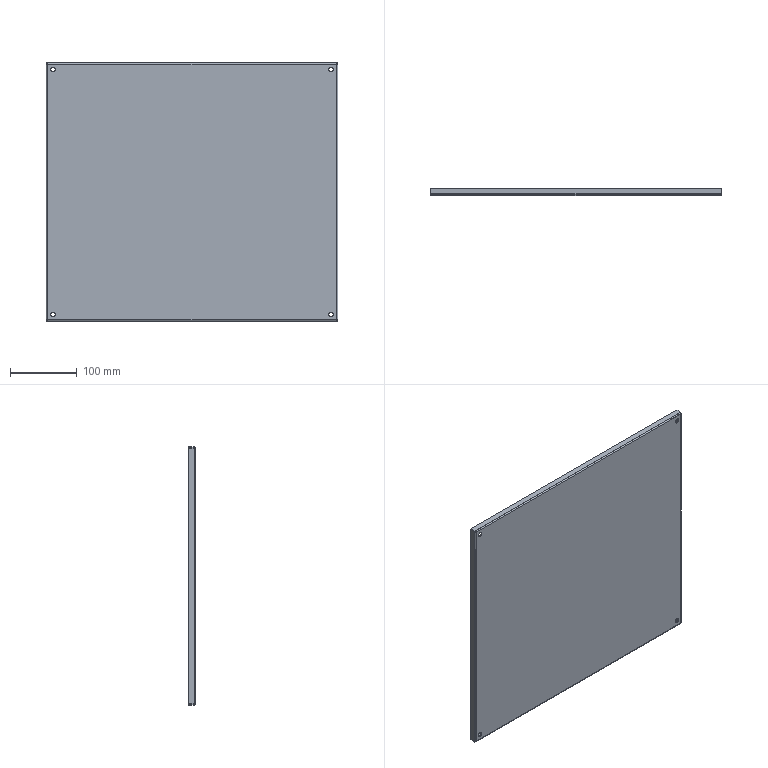Part | SolidWorks | features BaseBody 1 | 1 solid | 46 faces | box 436 x 10 x 386 mm | volume 272050 mm3 | plane 30 | cylinder 16 | commonest cylinder face diameters 7 x8 0.4 x4 3.4 x4
STEP:
#1=CARTESIAN_POINT('',(1238.,514.5,404.5));
#2=VERTEX_POINT('',#1);
#3=CARTESIAN_POINT('',(1238.,514.5,411.5));
#4=VERTEX_POINT('',#3);
#5=CARTESIAN_POINT('',(1238.,514.5,408.));
#6=DIRECTION('',(0.,1.,0.));
#7=DIRECTION('',(0.,0.,1.));
#8=AXIS2_PLACEMENT_3D('',#5,#6,#7);
#9=CIRCLE('',#8,3.5);
#10=EDGE_CURVE('',#2,#4,#9,.T.);
#11=ORIENTED_EDGE('',*,*,#10,.T.);
#12=CARTESIAN_POINT('',(1238.,513.,411.5));
#13=VERTEX_POINT('',#12);
#14=CARTESIAN_POINT('',(1238.,513.,411.5));
#15=DIRECTION('',(0.,-1.,0.));
#16=VECTOR('',#15,1000.);
#17=LINE('',#14,#16);
#18=EDGE_CURVE('',#4,#13,#17,.T.);
#19=ORIENTED_EDGE('',*,*,#18,.T.);
#20=CARTESIAN_POINT('',(1238.,513.,404.5));
#21=VERTEX_POINT('',#20);
#22=CARTESIAN_POINT('',(1238.,513.,408.));
#23=DIRECTION('',(0.,-1.,0.));
#24=DIRECTION('',(0.,0.,1.));
#25=AXIS2_PLACEMENT_3D('',#22,#23,#24);
#26=CIRCLE('',#25,3.5);
#27=EDGE_CURVE('',#13,#21,#26,.T.);
#28=ORIENTED_EDGE('',*,*,#27,.T.);
#29=CARTESIAN_POINT('',(1238.,513.,404.5));
#30=DIRECTION('',(0.,-1.,0.));
#31=VECTOR('',#30,1000.);
#32=LINE('',#29,#31);
#33=EDGE_CURVE('',#2,#21,#32,.T.);
#34=ORIENTED_EDGE('',*,*,#33,.F.);
#35=EDGE_LOOP('',(#11,#19,#28,#34));
#36=FACE_OUTER_BOUND('',#35,.T.);
#37=CARTESIAN_POINT('',(1238.,513.,408.));
#38=DIRECTION('',(0.,-1.,0.));
#39=DIRECTION('',(0.,0.,-1.));
#40=AXIS2_PLACEMENT_3D('',#37,#38,#39);
#41=CYLINDRICAL_SURFACE('',#40,3.5);
#42=ADVANCED_FACE('',(#36),#41,.F.);
#43=CARTESIAN_POINT('',(822.,514.5,38.5));
#44=VERTEX_POINT('',#43);
#45=CARTESIAN_POINT('',(822.,514.5,45.5));
#46=VERTEX_POINT('',#45);
#47=CARTESIAN_POINT('',(822.,514.5,42.));
#48=DIRECTION('',(0.,1.,0.));
#49=DIRECTION('',(0.,0.,1.));
#50=AXIS2_PLACEMENT_3D('',#47,#48,#49);
#51=CIRCLE('',#50,3.5);
#52=EDGE_CURVE('',#44,#46,#51,.T.);
#53=ORIENTED_EDGE('',*,*,#52,.T.);
#54=CARTESIAN_POINT('',(822.,513.,45.5));
#55=VERTEX_POINT('',#54);
#56=CARTESIAN_POINT('',(822.,513.,45.5));
#57=DIRECTION('',(0.,-1.,0.));
#58=VECTOR('',#57,1000.);
#59=LINE('',#56,#58);
#60=EDGE_CURVE('',#46,#55,#59,.T.);
#61=ORIENTED_EDGE('',*,*,#60,.T.);
#62=CARTESIAN_POINT('',(822.,513.,38.5));
#63=VERTEX_POINT('',#62);
#64=CARTESIAN_POINT('',(822.,513.,42.));
#65=DIRECTION('',(0.,-1.,0.));
#66=DIRECTION('',(0.,0.,1.));
#67=AXIS2_PLACEMENT_3D('',#64,#65,#66);
#68=CIRCLE('',#67,3.5);
#69=EDGE_CURVE('',#55,#63,#68,.T.);
#70=ORIENTED_EDGE('',*,*,#69,.T.);
#71=CARTESIAN_POINT('',(822.,513.,38.5));
#72=DIRECTION('',(0.,-1.,0.));
#73=VECTOR('',#72,1000.);
#74=LINE('',#71,#73);
#75=EDGE_CURVE('',#44,#63,#74,.T.);
#76=ORIENTED_EDGE('',*,*,#75,.F.);
#77=EDGE_LOOP('',(#53,#61,#70,#76));
#78=FACE_OUTER_BOUND('',#77,.T.);
#79=CARTESIAN_POINT('',(822.,513.,42.));
#80=DIRECTION('',(0.,-1.,0.));
#81=DIRECTION('',(0.,0.,-1.));
#82=AXIS2_PLACEMENT_3D('',#79,#80,#81);
#83=CYLINDRICAL_SURFACE('',#82,3.5);
#84=ADVANCED_FACE('',(#78),#83,.F.);
#85=CARTESIAN_POINT('',(822.,514.5,404.5));
#86=VERTEX_POINT('',#85);
#87=CARTESIAN_POINT('',(822.,514.5,411.5));
#88=VERTEX_POINT('',#87);
#89=CARTESIAN_POINT('',(822.,514.5,408.));
#90=DIRECTION('',(0.,1.,0.));
#91=DIRECTION('',(0.,0.,1.));
#92=AXIS2_PLACEMENT_3D('',#89,#90,#91);
#93=CIRCLE('',#92,3.5);
#94=EDGE_CURVE('',#86,#88,#93,.T.);
#95=ORIENTED_EDGE('',*,*,#94,.T.);
#96=CARTESIAN_POINT('',(822.,513.,411.5));
#97=VERTEX_POINT('',#96);
#98=CARTESIAN_POINT('',(822.,513.,411.5));
#99=DIRECTION('',(0.,-1.,0.));
#100=VECTOR('',#99,1000.);
#101=LINE('',#98,#100);
#102=EDGE_CURVE('',#88,#97,#101,.T.);
#103=ORIENTED_EDGE('',*,*,#102,.T.);
#104=CARTESIAN_POINT('',(822.,513.,404.5));
#105=VERTEX_POINT('',#104);
#106=CARTESIAN_POINT('',(822.,513.,408.));
#107=DIRECTION('',(0.,-1.,0.));
#108=DIRECTION('',(0.,0.,1.));
#109=AXIS2_PLACEMENT_3D('',#106,#107,#108);
#110=CIRCLE('',#109,3.5);
#111=EDGE_CURVE('',#97,#105,#110,.T.);
#112=ORIENTED_EDGE('',*,*,#111,.T.);
#113=CARTESIAN_POINT('',(822.,513.,404.5));
#114=DIRECTION('',(0.,-1.,0.));
#115=VECTOR('',#114,1000.);
#116=LINE('',#113,#115);
#117=EDGE_CURVE('',#86,#105,#116,.T.);
#118=ORIENTED_EDGE('',*,*,#117,.F.);
#119=EDGE_LOOP('',(#95,#103,#112,#118));
#120=FACE_OUTER_BOUND('',#119,.T.);
#121=CARTESIAN_POINT('',(822.,513.,408.));
#122=DIRECTION('',(0.,-1.,0.));
#123=DIRECTION('',(0.,0.,-1.));
#124=AXIS2_PLACEMENT_3D('',#121,#122,#123);
#125=CYLINDRICAL_SURFACE('',#124,3.5);
#126=ADVANCED_FACE('',(#120),#125,.F.);
#127=CARTESIAN_POINT('',(1238.,514.5,38.5));
#128=VERTEX_POINT('',#127);
#129=CARTESIAN_POINT('',(1238.,514.5,45.5));
#130=VERTEX_POINT('',#129);
#131=CARTESIAN_POINT('',(1238.,514.5,42.));
#132=DIRECTION('',(0.,1.,0.));
#133=DIRECTION('',(0.,0.,1.));
#134=AXIS2_PLACEMENT_3D('',#131,#132,#133);
#135=CIRCLE('',#134,3.5);
#136=EDGE_CURVE('',#128,#130,#135,.T.);
#137=ORIENTED_EDGE('',*,*,#136,.T.);
#138=CARTESIAN_POINT('',(1238.,513.,45.5));
#139=VERTEX_POINT('',#138);
#140=CARTESIAN_POINT('',(1238.,513.,45.5));
#141=DIRECTION('',(0.,-1.,0.));
#142=VECTOR('',#141,1000.);
#143=LINE('',#140,#142);
#144=EDGE_CURVE('',#130,#139,#143,.T.);
#145=ORIENTED_EDGE('',*,*,#144,.T.);
#146=CARTESIAN_POINT('',(1238.,513.,38.5));
#147=VERTEX_POINT('',#146);
#148=CARTESIAN_POINT('',(1238.,513.,42.));
#149=DIRECTION('',(0.,-1.,0.));
#150=DIRECTION('',(0.,0.,1.));
#151=AXIS2_PLACEMENT_3D('',#148,#149,#150);
#152=CIRCLE('',#151,3.5);
#153=EDGE_CURVE('',#139,#147,#152,.T.);
#154=ORIENTED_EDGE('',*,*,#153,.T.);
#155=CARTESIAN_POINT('',(1238.,513.,38.5));
#156=DIRECTION('',(0.,-1.,0.));
#157=VECTOR('',#156,1000.);
#158=LINE('',#155,#157);
#159=EDGE_CURVE('',#128,#147,#158,.T.);
#160=ORIENTED_EDGE('',*,*,#159,.F.);
#161=EDGE_LOOP('',(#137,#145,#154,#160));
#162=FACE_OUTER_BOUND('',#161,.T.);
#163=CARTESIAN_POINT('',(1238.,513.,42.));
#164=DIRECTION('',(0.,-1.,0.));
#165=DIRECTION('',(0.,0.,-1.));
#166=AXIS2_PLACEMENT_3D('',#163,#164,#165);
#167=CYLINDRICAL_SURFACE('',#166,3.5);
#168=ADVANCED_FACE('',(#162),#167,.F.);
#169=CARTESIAN_POINT('',(1246.5,514.7,416.));
#170=VERTEX_POINT('',#169);
#171=CARTESIAN_POINT('',(1246.3,514.5,416.));
#172=VERTEX_POINT('',#171);
#173=CARTESIAN_POINT('',(1246.3,514.7,416.));
#174=DIRECTION('',(0.,0.,-1.));
#175=DIRECTION('',(-1.,0.,0.));
#176=AXIS2_PLACEMENT_3D('',#173,#174,#175);
#177=CIRCLE('',#176,0.2);
#178=EDGE_CURVE('',#170,#172,#177,.T.);
#179=ORIENTED_EDGE('',*,*,#178,.F.);
#180=CARTESIAN_POINT('',(1246.5,514.7,34.));
#181=VERTEX_POINT('',#180);
#182=CARTESIAN_POINT('',(1246.5,514.7,421.));
#183=DIRECTION('',(0.,0.,1.));
#184=VECTOR('',#183,1000.);
#185=LINE('',#182,#184);
#186=EDGE_CURVE('',#181,#170,#185,.T.);
#187=ORIENTED_EDGE('',*,*,#186,.F.);
#188=CARTESIAN_POINT('',(1246.3,514.5,34.));
#189=VERTEX_POINT('',#188);
#190=CARTESIAN_POINT('',(1246.3,514.7,34.));
#191=DIRECTION('',(0.,0.,1.));
#192=DIRECTION('',(-1.,0.,0.));
#193=AXIS2_PLACEMENT_3D('',#190,#191,#192);
#194=CIRCLE('',#193,0.2);
#195=EDGE_CURVE('',#189,#181,#194,.T.);
#196=ORIENTED_EDGE('',*,*,#195,.F.);
#197=CARTESIAN_POINT('',(1246.3,514.5,421.));
#198=DIRECTION('',(0.,0.,-1.));
#199=VECTOR('',#198,1000.);
#200=LINE('',#197,#199);
#201=EDGE_CURVE('',#172,#189,#200,.T.);
#202=ORIENTED_EDGE('',*,*,#201,.F.);
#203=EDGE_LOOP('',(#179,#187,#196,#202));
#204=FACE_OUTER_BOUND('',#203,.T.);
#205=CARTESIAN_POINT('',(1246.3,514.7,1003.962));
#206=DIRECTION('',(0.,0.,-1.));
#207=DIRECTION('',(-1.,0.,0.));
#208=AXIS2_PLACEMENT_3D('',#205,#206,#207);
#209=CYLINDRICAL_SURFACE('',#208,0.2);
#210=ADVANCED_FACE('',(#204),#209,.F.);
#211=CARTESIAN_POINT('',(1248.,514.7,416.));
#212=VERTEX_POINT('',#211);
#213=CARTESIAN_POINT('',(1246.3,513.,416.));
#214=VERTEX_POINT('',#213);
#215=CARTESIAN_POINT('',(1246.3,514.7,416.));
#216=DIRECTION('',(0.,0.,-1.));
#217=DIRECTION('',(-1.,0.,0.));
#218=AXIS2_PLACEMENT_3D('',#215,#216,#217);
#219=CIRCLE('',#218,1.7);
#220=EDGE_CURVE('',#212,#214,#219,.T.);
#221=ORIENTED_EDGE('',*,*,#220,.T.);
#222=CARTESIAN_POINT('',(1246.3,513.,34.));
#223=VERTEX_POINT('',#222);
#224=CARTESIAN_POINT('',(1246.3,513.,421.));
#225=DIRECTION('',(0.,0.,-1.));
#226=VECTOR('',#225,1000.);
#227=LINE('',#224,#226);
#228=EDGE_CURVE('',#214,#223,#227,.T.);
#229=ORIENTED_EDGE('',*,*,#228,.T.);
#230=CARTESIAN_POINT('',(1248.,514.7,34.));
#231=VERTEX_POINT('',#230);
#232=CARTESIAN_POINT('',(1246.3,514.7,34.));
#233=DIRECTION('',(0.,0.,1.));
#234=DIRECTION('',(-1.,0.,0.));
#235=AXIS2_PLACEMENT_3D('',#232,#233,#234);
#236=CIRCLE('',#235,1.7);
#237=EDGE_CURVE('',#223,#231,#236,.T.);
#238=ORIENTED_EDGE('',*,*,#237,.T.);
#239=CARTESIAN_POINT('',(1248.,514.7,421.));
#240=DIRECTION('',(0.,0.,1.));
#241=VECTOR('',#240,1000.);
#242=LINE('',#239,#241);
#243=EDGE_CURVE('',#231,#212,#242,.T.);
#244=ORIENTED_EDGE('',*,*,#243,.T.);
#245=EDGE_LOOP('',(#221,#229,#238,#244));
#246=FACE_OUTER_BOUND('',#245,.T.);
#247=CARTESIAN_POINT('',(1246.3,514.7,1003.962));
#248=DIRECTION('',(0.,0.,-1.));
#249=DIRECTION('',(-1.,0.,0.));
#250=AXIS2_PLACEMENT_3D('',#247,#248,#249);
#251=CYLINDRICAL_SURFACE('',#250,1.7);
#252=ADVANCED_FACE('',(#246),#251,.T.);
#253=CARTESIAN_POINT('',(1246.,514.7,33.5));
#254=VERTEX_POINT('',#253);
#255=CARTESIAN_POINT('',(1246.,514.5,33.7));
#256=VERTEX_POINT('',#255);
#257=CARTESIAN_POINT('',(1246.,514.7,33.7));
#258=DIRECTION('',(-1.,0.,0.));
#259=DIRECTION('',(0.,0.,1.));
#260=AXIS2_PLACEMENT_3D('',#257,#258,#259);
#261=CIRCLE('',#260,0.2);
#262=EDGE_CURVE('',#254,#256,#261,.T.);
#263=ORIENTED_EDGE('',*,*,#262,.F.);
#264=CARTESIAN_POINT('',(814.,514.7,33.5));
#265=VERTEX_POINT('',#264);
#266=CARTESIAN_POINT('',(1251.,514.7,33.5));
#267=DIRECTION('',(1.,0.,0.));
#268=VECTOR('',#267,1000.);
#269=LINE('',#266,#268);
#270=EDGE_CURVE('',#265,#254,#269,.T.);
#271=ORIENTED_EDGE('',*,*,#270,.F.);
#272=CARTESIAN_POINT('',(814.,514.5,33.7));
#273=VERTEX_POINT('',#272);
#274=CARTESIAN_POINT('',(814.,514.7,33.7));
#275=DIRECTION('',(1.,0.,0.));
#276=DIRECTION('',(0.,0.,1.));
#277=AXIS2_PLACEMENT_3D('',#274,#275,#276);
#278=CIRCLE('',#277,0.2);
#279=EDGE_CURVE('',#273,#265,#278,.T.);
#280=ORIENTED_EDGE('',*,*,#279,.F.);
#281=CARTESIAN_POINT('',(1251.,514.5,33.7));
#282=DIRECTION('',(-1.,0.,0.));
#283=VECTOR('',#282,1000.);
#284=LINE('',#281,#283);
#285=EDGE_CURVE('',#256,#273,#284,.T.);
#286=ORIENTED_EDGE('',*,*,#285,.F.);
#287=EDGE_LOOP('',(#263,#271,#280,#286));
#288=FACE_OUTER_BOUND('',#287,.T.);
#289=CARTESIAN_POINT('',(1838.847,514.7,33.7));
#290=DIRECTION('',(-1.,0.,0.));
#291=DIRECTION('',(0.,0.,1.));
#292=AXIS2_PLACEMENT_3D('',#289,#290,#291);
#293=CYLINDRICAL_SURFACE('',#292,0.2);
#294=ADVANCED_FACE('',(#288),#293,.F.);
#295=CARTESIAN_POINT('',(1246.,514.7,32.));
#296=VERTEX_POINT('',#295);
#297=CARTESIAN_POINT('',(1246.,513.,33.7));
#298=VERTEX_POINT('',#297);
#299=CARTESIAN_POINT('',(1246.,514.7,33.7));
#300=DIRECTION('',(-1.,0.,0.));
#301=DIRECTION('',(0.,0.,1.));
#302=AXIS2_PLACEMENT_3D('',#299,#300,#301);
#303=CIRCLE('',#302,1.7);
#304=EDGE_CURVE('',#296,#298,#303,.T.);
#305=ORIENTED_EDGE('',*,*,#304,.T.);
#306=CARTESIAN_POINT('',(814.,513.,33.7));
#307=VERTEX_POINT('',#306);
#308=CARTESIAN_POINT('',(1251.,513.,33.7));
#309=DIRECTION('',(-1.,0.,0.));
#310=VECTOR('',#309,1000.);
#311=LINE('',#308,#310);
#312=EDGE_CURVE('',#298,#307,#311,.T.);
#313=ORIENTED_EDGE('',*,*,#312,.T.);
#314=CARTESIAN_POINT('',(814.,514.7,32.));
#315=VERTEX_POINT('',#314);
#316=CARTESIAN_POINT('',(814.,514.7,33.7));
#317=DIRECTION('',(1.,0.,0.));
#318=DIRECTION('',(0.,0.,1.));
#319=AXIS2_PLACEMENT_3D('',#316,#317,#318);
#320=CIRCLE('',#319,1.7);
#321=EDGE_CURVE('',#307,#315,#320,.T.);
#322=ORIENTED_EDGE('',*,*,#321,.T.);
#323=CARTESIAN_POINT('',(1251.,514.7,32.));
#324=DIRECTION('',(1.,0.,0.));
#325=VECTOR('',#324,1000.);
#326=LINE('',#323,#325);
#327=EDGE_CURVE('',#315,#296,#326,.T.);
#328=ORIENTED_EDGE('',*,*,#327,.T.);
#329=EDGE_LOOP('',(#305,#313,#322,#328));
#330=FACE_OUTER_BOUND('',#329,.T.);
#331=CARTESIAN_POINT('',(1838.847,514.7,33.7));
#332=DIRECTION('',(-1.,0.,0.));
#333=DIRECTION('',(0.,0.,1.));
#334=AXIS2_PLACEMENT_3D('',#331,#332,#333);
#335=CYLINDRICAL_SURFACE('',#334,1.7);
#336=ADVANCED_FACE('',(#330),#335,.T.);
#337=CARTESIAN_POINT('',(813.5,514.7,34.));
#338=VERTEX_POINT('',#337);
#339=CARTESIAN_POINT('',(813.7,514.5,34.));
#340=VERTEX_POINT('',#339);
#341=CARTESIAN_POINT('',(813.7,514.7,34.));
#342=DIRECTION('',(0.,0.,1.));
#343=DIRECTION('',(1.,0.,0.));
#344=AXIS2_PLACEMENT_3D('',#341,#342,#343);
#345=CIRCLE('',#344,0.2);
#346=EDGE_CURVE('',#338,#340,#345,.T.);
#347=ORIENTED_EDGE('',*,*,#346,.F.);
#348=CARTESIAN_POINT('',(813.5,514.7,416.));
#349=VERTEX_POINT('',#348);
#350=CARTESIAN_POINT('',(813.5,514.7,29.));
#351=DIRECTION('',(0.,0.,-1.));
#352=VECTOR('',#351,1000.);
#353=LINE('',#350,#352);
#354=EDGE_CURVE('',#349,#338,#353,.T.);
#355=ORIENTED_EDGE('',*,*,#354,.F.);
#356=CARTESIAN_POINT('',(813.7,514.5,416.));
#357=VERTEX_POINT('',#356);
#358=CARTESIAN_POINT('',(813.7,514.7,416.));
#359=DIRECTION('',(0.,0.,-1.));
#360=DIRECTION('',(1.,0.,0.));
#361=AXIS2_PLACEMENT_3D('',#358,#359,#360);
#362=CIRCLE('',#361,0.2);
#363=EDGE_CURVE('',#357,#349,#362,.T.);
#364=ORIENTED_EDGE('',*,*,#363,.F.);
#365=CARTESIAN_POINT('',(813.7,514.5,29.));
#366=DIRECTION('',(0.,0.,1.));
#367=VECTOR('',#366,1000.);
#368=LINE('',#365,#367);
#369=EDGE_CURVE('',#340,#357,#368,.T.);
#370=ORIENTED_EDGE('',*,*,#369,.F.);
#371=EDGE_LOOP('',(#347,#355,#364,#370));
#372=FACE_OUTER_BOUND('',#371,.T.);
#373=CARTESIAN_POINT('',(813.7,514.7,-564.401));
#374=DIRECTION('',(0.,0.,1.));
#375=DIRECTION('',(1.,0.,0.));
#376=AXIS2_PLACEMENT_3D('',#373,#374,#375);
#377=CYLINDRICAL_SURFACE('',#376,0.2);
#378=ADVANCED_FACE('',(#372),#377,.F.);
#379=CARTESIAN_POINT('',(812.,514.7,34.));
#380=VERTEX_POINT('',#379);
#381=CARTESIAN_POINT('',(813.7,513.,34.));
#382=VERTEX_POINT('',#381);
#383=CARTESIAN_POINT('',(813.7,514.7,34.));
#384=DIRECTION('',(0.,0.,1.));
#385=DIRECTION('',(1.,0.,0.));
#386=AXIS2_PLACEMENT_3D('',#383,#384,#385);
#387=CIRCLE('',#386,1.7);
#388=EDGE_CURVE('',#380,#382,#387,.T.);
#389=ORIENTED_EDGE('',*,*,#388,.T.);
#390=CARTESIAN_POINT('',(813.7,513.,416.));
#391=VERTEX_POINT('',#390);
#392=CARTESIAN_POINT('',(813.7,513.,29.));
#393=DIRECTION('',(0.,0.,1.));
#394=VECTOR('',#393,1000.);
#395=LINE('',#392,#394);
#396=EDGE_CURVE('',#382,#391,#395,.T.);
#397=ORIENTED_EDGE('',*,*,#396,.T.);
#398=CARTESIAN_POINT('',(812.,514.7,416.));
#399=VERTEX_POINT('',#398);
#400=CARTESIAN_POINT('',(813.7,514.7,416.));
#401=DIRECTION('',(0.,0.,-1.));
#402=DIRECTION('',(1.,0.,0.));
#403=AXIS2_PLACEMENT_3D('',#400,#401,#402);
#404=CIRCLE('',#403,1.7);
#405=EDGE_CURVE('',#391,#399,#404,.T.);
#406=ORIENTED_EDGE('',*,*,#405,.T.);
#407=CARTESIAN_POINT('',(812.,514.7,29.));
#408=DIRECTION('',(0.,0.,-1.));
#409=VECTOR('',#408,1000.);
#410=LINE('',#407,#409);
#411=EDGE_CURVE('',#399,#380,#410,.T.);
#412=ORIENTED_EDGE('',*,*,#411,.T.);
#413=EDGE_LOOP('',(#389,#397,#406,#412));
#414=FACE_OUTER_BOUND('',#413,.T.);
#415=CARTESIAN_POINT('',(813.7,514.7,-564.401));
#416=DIRECTION('',(0.,0.,1.));
#417=DIRECTION('',(1.,0.,0.));
#418=AXIS2_PLACEMENT_3D('',#415,#416,#417);
#419=CYLINDRICAL_SURFACE('',#418,1.7);
#420=ADVANCED_FACE('',(#414),#419,.T.);
#421=CARTESIAN_POINT('',(814.,514.7,416.5));
#422=VERTEX_POINT('',#421);
#423=CARTESIAN_POINT('',(814.,514.5,416.3));
#424=VERTEX_POINT('',#423);
#425=CARTESIAN_POINT('',(814.,514.7,416.3));
#426=DIRECTION('',(1.,0.,0.));
#427=DIRECTION('',(0.,0.,-1.));
#428=AXIS2_PLACEMENT_3D('',#425,#426,#427);
#429=CIRCLE('',#428,0.2);
#430=EDGE_CURVE('',#422,#424,#429,.T.);
#431=ORIENTED_EDGE('',*,*,#430,.F.);
#432=CARTESIAN_POINT('',(1246.,514.7,416.5));
#433=VERTEX_POINT('',#432);
#434=CARTESIAN_POINT('',(809.,514.7,416.5));
#435=DIRECTION('',(-1.,0.,0.));
#436=VECTOR('',#435,1000.);
#437=LINE('',#434,#436);
#438=EDGE_CURVE('',#433,#422,#437,.T.);
#439=ORIENTED_EDGE('',*,*,#438,.F.);
#440=CARTESIAN_POINT('',(1246.,514.5,416.3));
#441=VERTEX_POINT('',#440);
#442=CARTESIAN_POINT('',(1246.,514.7,416.3));
#443=DIRECTION('',(-1.,0.,0.));
#444=DIRECTION('',(0.,0.,-1.));
#445=AXIS2_PLACEMENT_3D('',#442,#443,#444);
#446=CIRCLE('',#445,0.2);
#447=EDGE_CURVE('',#441,#433,#446,.T.);
#448=ORIENTED_EDGE('',*,*,#447,.F.);
#449=CARTESIAN_POINT('',(809.,514.5,416.3));
#450=DIRECTION('',(1.,0.,0.));
#451=VECTOR('',#450,1000.);
#452=LINE('',#449,#451);
#453=EDGE_CURVE('',#424,#441,#452,.T.);
#454=ORIENTED_EDGE('',*,*,#453,.F.);
#455=EDGE_LOOP('',(#431,#439,#448,#454));
#456=FACE_OUTER_BOUND('',#455,.T.);
#457=CARTESIAN_POINT('',(210.789,514.7,416.3));
#458=DIRECTION('',(1.,0.,0.));
#459=DIRECTION('',(0.,0.,-1.));
#460=AXIS2_PLACEMENT_3D('',#457,#458,#459);
#461=CYLINDRICAL_SURFACE('',#460,0.2);
#462=ADVANCED_FACE('',(#456),#461,.F.);
#463=CARTESIAN_POINT('',(814.,514.7,418.));
#464=VERTEX_POINT('',#463);
#465=CARTESIAN_POINT('',(814.,513.,416.3));
#466=VERTEX_POINT('',#465);
#467=CARTESIAN_POINT('',(814.,514.7,416.3));
#468=DIRECTION('',(1.,0.,0.));
#469=DIRECTION('',(0.,0.,-1.));
#470=AXIS2_PLACEMENT_3D('',#467,#468,#469);
#471=CIRCLE('',#470,1.7);
#472=EDGE_CURVE('',#464,#466,#471,.T.);
#473=ORIENTED_EDGE('',*,*,#472,.T.);
#474=CARTESIAN_POINT('',(1246.,513.,416.3));
#475=VERTEX_POINT('',#474);
#476=CARTESIAN_POINT('',(809.,513.,416.3));
#477=DIRECTION('',(1.,0.,0.));
#478=VECTOR('',#477,1000.);
#479=LINE('',#476,#478);
#480=EDGE_CURVE('',#466,#475,#479,.T.);
#481=ORIENTED_EDGE('',*,*,#480,.T.);
#482=CARTESIAN_POINT('',(1246.,514.7,418.));
#483=VERTEX_POINT('',#482);
#484=CARTESIAN_POINT('',(1246.,514.7,416.3));
#485=DIRECTION('',(-1.,0.,0.));
#486=DIRECTION('',(0.,0.,-1.));
#487=AXIS2_PLACEMENT_3D('',#484,#485,#486);
#488=CIRCLE('',#487,1.7);
#489=EDGE_CURVE('',#475,#483,#488,.T.);
#490=ORIENTED_EDGE('',*,*,#489,.T.);
#491=CARTESIAN_POINT('',(809.,514.7,418.));
#492=DIRECTION('',(-1.,0.,0.));
#493=VECTOR('',#492,1000.);
#494=LINE('',#491,#493);
#495=EDGE_CURVE('',#483,#464,#494,.T.);
#496=ORIENTED_EDGE('',*,*,#495,.T.);
#497=EDGE_LOOP('',(#473,#481,#490,#496));
#498=FACE_OUTER_BOUND('',#497,.T.);
#499=CARTESIAN_POINT('',(210.789,514.7,416.3));
#500=DIRECTION('',(1.,0.,0.));
#501=DIRECTION('',(0.,0.,-1.));
#502=AXIS2_PLACEMENT_3D('',#499,#500,#501);
#503=CYLINDRICAL_SURFACE('',#502,1.7);
#504=ADVANCED_FACE('',(#498),#503,.T.);
#505=CARTESIAN_POINT('',(1246.,514.5,416.));
#506=VERTEX_POINT('',#505);
#507=CARTESIAN_POINT('',(1246.,514.5,-5.));
#508=DIRECTION('',(0.,0.,-1.));
#509=VECTOR('',#508,1000.);
#510=LINE('',#507,#509);
#511=EDGE_CURVE('',#441,#506,#510,.T.);
#512=ORIENTED_EDGE('',*,*,#511,.F.);
#513=ORIENTED_EDGE('',*,*,#447,.T.);
#514=CARTESIAN_POINT('',(1246.,514.7,-454.158));
#515=DIRECTION('',(0.,0.,1.));
#516=VECTOR('',#515,1000.);
#517=LINE('',#514,#516);
#518=EDGE_CURVE('',#433,#483,#517,.T.);
#519=ORIENTED_EDGE('',*,*,#518,.T.);
#520=ORIENTED_EDGE('',*,*,#489,.F.);
#521=CARTESIAN_POINT('',(1246.,513.,416.));
#522=VERTEX_POINT('',#521);
#523=CARTESIAN_POINT('',(1246.,513.,-5.));
#524=DIRECTION('',(0.,0.,-1.));
#525=VECTOR('',#524,1000.);
#526=LINE('',#523,#525);
#527=EDGE_CURVE('',#475,#522,#526,.T.);
#528=ORIENTED_EDGE('',*,*,#527,.T.);
#529=CARTESIAN_POINT('',(1246.,1668.033,416.));
#530=DIRECTION('',(0.,-1.,0.));
#531=VECTOR('',#530,1000.);
#532=LINE('',#529,#531);
#533=EDGE_CURVE('',#506,#522,#532,.T.);
#534=ORIENTED_EDGE('',*,*,#533,.F.);
#535=EDGE_LOOP('',(#512,#513,#519,#520,#528,#534));
#536=FACE_OUTER_BOUND('',#535,.T.);
#537=CARTESIAN_POINT('',(1246.,1668.033,-5.));
#538=DIRECTION('',(-1.,0.,0.));
#539=DIRECTION('',(0.,1.,0.));
#540=AXIS2_PLACEMENT_3D('',#537,#538,#539);
#541=PLANE('',#540);
#542=ADVANCED_FACE('',(#536),#541,.F.);
#543=CARTESIAN_POINT('',(814.,514.5,416.));
#544=VERTEX_POINT('',#543);
#545=CARTESIAN_POINT('',(814.,513.,416.));
#546=VERTEX_POINT('',#545);
#547=CARTESIAN_POINT('',(814.,1668.033,416.));
#548=DIRECTION('',(0.,-1.,0.));
#549=VECTOR('',#548,1000.);
#550=LINE('',#547,#549);
#551=EDGE_CURVE('',#544,#546,#550,.T.);
#552=ORIENTED_EDGE('',*,*,#551,.T.);
#553=CARTESIAN_POINT('',(814.,513.,-5.));
#554=DIRECTION('',(0.,0.,1.));
#555=VECTOR('',#554,1000.);
#556=LINE('',#553,#555);
#557=EDGE_CURVE('',#546,#466,#556,.T.);
#558=ORIENTED_EDGE('',*,*,#557,.T.);
#559=ORIENTED_EDGE('',*,*,#472,.F.);
#560=CARTESIAN_POINT('',(814.,514.7,-454.158));
#561=DIRECTION('',(0.,0.,1.));
#562=VECTOR('',#561,1000.);
#563=LINE('',#560,#562);
#564=EDGE_CURVE('',#422,#464,#563,.T.);
#565=ORIENTED_EDGE('',*,*,#564,.F.);
#566=ORIENTED_EDGE('',*,*,#430,.T.);
#567=CARTESIAN_POINT('',(814.,514.5,-5.));
#568=DIRECTION('',(0.,0.,1.));
#569=VECTOR('',#568,1000.);
#570=LINE('',#567,#569);
#571=EDGE_CURVE('',#544,#424,#570,.T.);
#572=ORIENTED_EDGE('',*,*,#571,.F.);
#573=EDGE_LOOP('',(#552,#558,#559,#565,#566,#572));
#574=FACE_OUTER_BOUND('',#573,.T.);
#575=CARTESIAN_POINT('',(814.,1668.033,-5.));
#576=DIRECTION('',(1.,0.,0.));
#577=DIRECTION('',(0.,0.,-1.));
#578=AXIS2_PLACEMENT_3D('',#575,#576,#577);
#579=PLANE('',#578);
#580=ADVANCED_FACE('',(#574),#579,.F.);
#581=CARTESIAN_POINT('',(814.,514.5,34.));
#582=VERTEX_POINT('',#581);
#583=CARTESIAN_POINT('',(814.,514.5,5.));
#584=DIRECTION('',(0.,0.,1.));
#585=VECTOR('',#584,1000.);
#586=LINE('',#583,#585);
#587=EDGE_CURVE('',#273,#582,#586,.T.);
#588=ORIENTED_EDGE('',*,*,#587,.F.);
#589=ORIENTED_EDGE('',*,*,#279,.T.);
#590=CARTESIAN_POINT('',(814.,514.7,904.158));
#591=DIRECTION('',(0.,0.,-1.));
#592=VECTOR('',#591,1000.);
#593=LINE('',#590,#592);
#594=EDGE_CURVE('',#265,#315,#593,.T.);
#595=ORIENTED_EDGE('',*,*,#594,.T.);
#596=ORIENTED_EDGE('',*,*,#321,.F.);
#597=CARTESIAN_POINT('',(814.,513.,34.));
#598=VERTEX_POINT('',#597);
#599=CARTESIAN_POINT('',(814.,513.,5.));
#600=DIRECTION('',(0.,0.,1.));
#601=VECTOR('',#600,1000.);
#602=LINE('',#599,#601);
#603=EDGE_CURVE('',#307,#598,#602,.T.);
#604=ORIENTED_EDGE('',*,*,#603,.T.);
#605=CARTESIAN_POINT('',(814.,1668.033,34.));
#606=DIRECTION('',(0.,-1.,0.));
#607=VECTOR('',#606,1000.);
#608=LINE('',#605,#607);
#609=EDGE_CURVE('',#582,#598,#608,.T.);
#610=ORIENTED_EDGE('',*,*,#609,.F.);
#611=EDGE_LOOP('',(#588,#589,#595,#596,#604,#610));
#612=FACE_OUTER_BOUND('',#611,.T.);
#613=CARTESIAN_POINT('',(814.,1668.033,5.));
#614=DIRECTION('',(1.,0.,0.));
#615=DIRECTION('',(0.,0.,1.));
#616=AXIS2_PLACEMENT_3D('',#613,#614,#615);
#617=PLANE('',#616);
#618=ADVANCED_FACE('',(#612),#617,.F.);
#619=CARTESIAN_POINT('',(1246.,514.5,34.));
#620=VERTEX_POINT('',#619);
#621=CARTESIAN_POINT('',(1246.,513.,34.));
#622=VERTEX_POINT('',#621);
#623=CARTESIAN_POINT('',(1246.,1668.033,34.));
#624=DIRECTION('',(0.,-1.,0.));
#625=VECTOR('',#624,1000.);
#626=LINE('',#623,#625);
#627=EDGE_CURVE('',#620,#622,#626,.T.);
#628=ORIENTED_EDGE('',*,*,#627,.T.);
#629=CARTESIAN_POINT('',(1246.,513.,5.));
#630=DIRECTION('',(0.,0.,-1.));
#631=VECTOR('',#630,1000.);
#632=LINE('',#629,#631);
#633=EDGE_CURVE('',#622,#298,#632,.T.);
#634=ORIENTED_EDGE('',*,*,#633,.T.);
#635=ORIENTED_EDGE('',*,*,#304,.F.);
#636=CARTESIAN_POINT('',(1246.,514.7,904.158));
#637=DIRECTION('',(0.,0.,-1.));
#638=VECTOR('',#637,1000.);
#639=LINE('',#636,#638);
#640=EDGE_CURVE('',#254,#296,#639,.T.);
#641=ORIENTED_EDGE('',*,*,#640,.F.);
#642=ORIENTED_EDGE('',*,*,#262,.T.);
#643=CARTESIAN_POINT('',(1246.,514.5,5.));
#644=DIRECTION('',(0.,0.,-1.));
#645=VECTOR('',#644,1000.);
#646=LINE('',#643,#645);
#647=EDGE_CURVE('',#620,#256,#646,.T.);
#648=ORIENTED_EDGE('',*,*,#647,.F.);
#649=EDGE_LOOP('',(#628,#634,#635,#641,#642,#648));
#650=FACE_OUTER_BOUND('',#649,.T.);
#651=CARTESIAN_POINT('',(1246.,1668.033,5.));
#652=DIRECTION('',(-1.,0.,0.));
#653=DIRECTION('',(0.,1.,0.));
#654=AXIS2_PLACEMENT_3D('',#651,#652,#653);
#655=PLANE('',#654);
#656=ADVANCED_FACE('',(#650),#655,.F.);
#657=ORIENTED_EDGE('',*,*,#136,.F.);
#658=CARTESIAN_POINT('',(1238.,514.5,42.));
#659=DIRECTION('',(0.,1.,0.));
#660=DIRECTION('',(0.,0.,1.));
#661=AXIS2_PLACEMENT_3D('',#658,#659,#660);
#662=CIRCLE('',#661,3.5);
#663=EDGE_CURVE('',#130,#128,#662,.T.);
#664=ORIENTED_EDGE('',*,*,#663,.F.);
#665=EDGE_LOOP('',(#657,#664));
#666=FACE_BOUND('',#665,.T.);
#667=ORIENTED_EDGE('',*,*,#94,.F.);
#668=CARTESIAN_POINT('',(822.,514.5,408.));
#669=DIRECTION('',(0.,1.,0.));
#670=DIRECTION('',(0.,0.,1.));
#671=AXIS2_PLACEMENT_3D('',#668,#669,#670);
#672=CIRCLE('',#671,3.5);
#673=EDGE_CURVE('',#88,#86,#672,.T.);
#674=ORIENTED_EDGE('',*,*,#673,.F.);
#675=EDGE_LOOP('',(#667,#674));
#676=FACE_BOUND('',#675,.T.);
#677=ORIENTED_EDGE('',*,*,#52,.F.);
#678=CARTESIAN_POINT('',(822.,514.5,42.));
#679=DIRECTION('',(0.,1.,0.));
#680=DIRECTION('',(0.,0.,1.));
#681=AXIS2_PLACEMENT_3D('',#678,#679,#680);
#682=CIRCLE('',#681,3.5);
#683=EDGE_CURVE('',#46,#44,#682,.T.);
#684=ORIENTED_EDGE('',*,*,#683,.F.);
#685=EDGE_LOOP('',(#677,#684));
#686=FACE_BOUND('',#685,.T.);
#687=ORIENTED_EDGE('',*,*,#10,.F.);
#688=CARTESIAN_POINT('',(1238.,514.5,408.));
#689=DIRECTION('',(0.,1.,0.));
#690=DIRECTION('',(0.,0.,1.));
#691=AXIS2_PLACEMENT_3D('',#688,#689,#690);
#692=CIRCLE('',#691,3.5);
#693=EDGE_CURVE('',#4,#2,#692,.T.);
#694=ORIENTED_EDGE('',*,*,#693,.F.);
#695=EDGE_LOOP('',(#687,#694));
#696=FACE_BOUND('',#695,.T.);
#697=CARTESIAN_POINT('',(-5.,514.5,416.));
#698=DIRECTION('',(1.,0.,0.));
#699=VECTOR('',#698,1000.);
#700=LINE('',#697,#699);
#701=EDGE_CURVE('',#506,#172,#700,.T.);
#702=ORIENTED_EDGE('',*,*,#701,.T.);
#703=ORIENTED_EDGE('',*,*,#201,.T.);
#704=CARTESIAN_POINT('',(-5.,514.5,34.));
#705=DIRECTION('',(-1.,0.,0.));
#706=VECTOR('',#705,1000.);
#707=LINE('',#704,#706);
#708=EDGE_CURVE('',#189,#620,#707,.T.);
#709=ORIENTED_EDGE('',*,*,#708,.T.);
#710=ORIENTED_EDGE('',*,*,#647,.T.);
#711=ORIENTED_EDGE('',*,*,#285,.T.);
#712=ORIENTED_EDGE('',*,*,#587,.T.);
#713=CARTESIAN_POINT('',(5.,514.5,34.));
#714=DIRECTION('',(-1.,0.,0.));
#715=VECTOR('',#714,1000.);
#716=LINE('',#713,#715);
#717=EDGE_CURVE('',#582,#340,#716,.T.);
#718=ORIENTED_EDGE('',*,*,#717,.T.);
#719=ORIENTED_EDGE('',*,*,#369,.T.);
#720=CARTESIAN_POINT('',(5.,514.5,416.));
#721=DIRECTION('',(1.,0.,0.));
#722=VECTOR('',#721,1000.);
#723=LINE('',#720,#722);
#724=EDGE_CURVE('',#357,#544,#723,.T.);
#725=ORIENTED_EDGE('',*,*,#724,.T.);
#726=ORIENTED_EDGE('',*,*,#571,.T.);
#727=ORIENTED_EDGE('',*,*,#453,.T.);
#728=ORIENTED_EDGE('',*,*,#511,.T.);
#729=EDGE_LOOP('',(#702,#703,#709,#710,#711,#712,#718,#719,#725,#726,#727,#728));
#730=FACE_OUTER_BOUND('',#729,.T.);
#731=CARTESIAN_POINT('',(0.,514.5,0.));
#732=DIRECTION('',(0.,1.,0.));
#733=DIRECTION('',(1.,0.,0.));
#734=AXIS2_PLACEMENT_3D('',#731,#732,#733);
#735=PLANE('',#734);
#736=ADVANCED_FACE('',(#666,#676,#686,#696,#730),#735,.T.);
#737=CARTESIAN_POINT('',(1238.,513.,408.));
#738=DIRECTION('',(0.,-1.,0.));
#739=DIRECTION('',(0.,0.,1.));
#740=AXIS2_PLACEMENT_3D('',#737,#738,#739);
#741=CIRCLE('',#740,3.5);
#742=EDGE_CURVE('',#21,#13,#741,.T.);
#743=ORIENTED_EDGE('',*,*,#742,.F.);
#744=ORIENTED_EDGE('',*,*,#27,.F.);
#745=EDGE_LOOP('',(#743,#744));
#746=FACE_BOUND('',#745,.T.);
#747=CARTESIAN_POINT('',(1238.,513.,42.));
#748=DIRECTION('',(0.,-1.,0.));
#749=DIRECTION('',(0.,0.,1.));
#750=AXIS2_PLACEMENT_3D('',#747,#748,#749);
#751=CIRCLE('',#750,3.5);
#752=EDGE_CURVE('',#147,#139,#751,.T.);
#753=ORIENTED_EDGE('',*,*,#752,.F.);
#754=ORIENTED_EDGE('',*,*,#153,.F.);
#755=EDGE_LOOP('',(#753,#754));
#756=FACE_BOUND('',#755,.T.);
#757=CARTESIAN_POINT('',(822.,513.,408.));
#758=DIRECTION('',(0.,-1.,0.));
#759=DIRECTION('',(0.,0.,1.));
#760=AXIS2_PLACEMENT_3D('',#757,#758,#759);
#761=CIRCLE('',#760,3.5);
#762=EDGE_CURVE('',#105,#97,#761,.T.);
#763=ORIENTED_EDGE('',*,*,#762,.F.);
#764=ORIENTED_EDGE('',*,*,#111,.F.);
#765=EDGE_LOOP('',(#763,#764));
#766=FACE_BOUND('',#765,.T.);
#767=CARTESIAN_POINT('',(822.,513.,42.));
#768=DIRECTION('',(0.,-1.,0.));
#769=DIRECTION('',(0.,0.,1.));
#770=AXIS2_PLACEMENT_3D('',#767,#768,#769);
#771=CIRCLE('',#770,3.5);
#772=EDGE_CURVE('',#63,#55,#771,.T.);
#773=ORIENTED_EDGE('',*,*,#772,.F.);
#774=ORIENTED_EDGE('',*,*,#69,.F.);
#775=EDGE_LOOP('',(#773,#774));
#776=FACE_BOUND('',#775,.T.);
#777=ORIENTED_EDGE('',*,*,#228,.F.);
#778=CARTESIAN_POINT('',(-5.,513.,416.));
#779=DIRECTION('',(1.,0.,0.));
#780=VECTOR('',#779,1000.);
#781=LINE('',#778,#780);
#782=EDGE_CURVE('',#522,#214,#781,.T.);
#783=ORIENTED_EDGE('',*,*,#782,.F.);
#784=ORIENTED_EDGE('',*,*,#527,.F.);
#785=ORIENTED_EDGE('',*,*,#480,.F.);
#786=ORIENTED_EDGE('',*,*,#557,.F.);
#787=CARTESIAN_POINT('',(5.,513.,416.));
#788=DIRECTION('',(1.,0.,0.));
#789=VECTOR('',#788,1000.);
#790=LINE('',#787,#789);
#791=EDGE_CURVE('',#391,#546,#790,.T.);
#792=ORIENTED_EDGE('',*,*,#791,.F.);
#793=ORIENTED_EDGE('',*,*,#396,.F.);
#794=CARTESIAN_POINT('',(5.,513.,34.));
#795=DIRECTION('',(-1.,0.,0.));
#796=VECTOR('',#795,1000.);
#797=LINE('',#794,#796);
#798=EDGE_CURVE('',#598,#382,#797,.T.);
#799=ORIENTED_EDGE('',*,*,#798,.F.);
#800=ORIENTED_EDGE('',*,*,#603,.F.);
#801=ORIENTED_EDGE('',*,*,#312,.F.);
#802=ORIENTED_EDGE('',*,*,#633,.F.);
#803=CARTESIAN_POINT('',(-5.,513.,34.));
#804=DIRECTION('',(-1.,0.,0.));
#805=VECTOR('',#804,1000.);
#806=LINE('',#803,#805);
#807=EDGE_CURVE('',#223,#622,#806,.T.);
#808=ORIENTED_EDGE('',*,*,#807,.F.);
#809=EDGE_LOOP('',(#777,#783,#784,#785,#786,#792,#793,#799,#800,#801,#802,#808));
#810=FACE_OUTER_BOUND('',#809,.T.);
#811=CARTESIAN_POINT('',(0.,513.,0.));
#812=DIRECTION('',(0.,1.,0.));
#813=DIRECTION('',(1.,0.,0.));
#814=AXIS2_PLACEMENT_3D('',#811,#812,#813);
#815=PLANE('',#814);
#816=ADVANCED_FACE('',(#746,#756,#766,#776,#810),#815,.F.);
#817=CARTESIAN_POINT('',(812.,523.,416.5));
#818=VERTEX_POINT('',#817);
#819=CARTESIAN_POINT('',(1248.,523.,416.5));
#820=VERTEX_POINT('',#819);
#821=CARTESIAN_POINT('',(808.5,523.,416.5));
#822=DIRECTION('',(1.,0.,0.));
#823=VECTOR('',#822,1000.);
#824=LINE('',#821,#823);
#825=EDGE_CURVE('',#818,#820,#824,.T.);
#826=ORIENTED_EDGE('',*,*,#825,.T.);
#827=CARTESIAN_POINT('',(1248.,514.7,416.5));
#828=VERTEX_POINT('',#827);
#829=CARTESIAN_POINT('',(1248.,-79.198,416.5));
#830=DIRECTION('',(0.,-1.,0.));
#831=VECTOR('',#830,1000.);
#832=LINE('',#829,#831);
#833=EDGE_CURVE('',#820,#828,#832,.T.);
#834=ORIENTED_EDGE('',*,*,#833,.T.);
#835=CARTESIAN_POINT('',(1248.002,514.7,416.5));
#836=DIRECTION('',(-1.,0.,0.));
#837=VECTOR('',#836,1000.);
#838=LINE('',#835,#837);
#839=EDGE_CURVE('',#828,#433,#838,.T.);
#840=ORIENTED_EDGE('',*,*,#839,.T.);
#841=ORIENTED_EDGE('',*,*,#438,.T.);
#842=CARTESIAN_POINT('',(812.,514.7,416.5));
#843=VERTEX_POINT('',#842);
#844=CARTESIAN_POINT('',(811.998,514.7,416.5));
#845=DIRECTION('',(1.,0.,0.));
#846=VECTOR('',#845,1000.);
#847=LINE('',#844,#846);
#848=EDGE_CURVE('',#843,#422,#847,.T.);
#849=ORIENTED_EDGE('',*,*,#848,.F.);
#850=CARTESIAN_POINT('',(812.,-79.198,416.5));
#851=DIRECTION('',(0.,1.,0.));
#852=VECTOR('',#851,1000.);
#853=LINE('',#850,#852);
#854=EDGE_CURVE('',#843,#818,#853,.T.);
#855=ORIENTED_EDGE('',*,*,#854,.T.);
#856=EDGE_LOOP('',(#826,#834,#840,#841,#849,#855));
#857=FACE_OUTER_BOUND('',#856,.T.);
#858=CARTESIAN_POINT('',(808.5,-79.198,416.5));
#859=DIRECTION('',(0.,0.,1.));
#860=DIRECTION('',(1.,0.,0.));
#861=AXIS2_PLACEMENT_3D('',#858,#859,#860);
#862=PLANE('',#861);
#863=ADVANCED_FACE('',(#857),#862,.F.);
#864=CARTESIAN_POINT('',(1248.,514.7,418.));
#865=VERTEX_POINT('',#864);
#866=CARTESIAN_POINT('',(1248.002,514.7,418.));
#867=DIRECTION('',(-1.,0.,0.));
#868=VECTOR('',#867,1000.);
#869=LINE('',#866,#868);
#870=EDGE_CURVE('',#865,#483,#869,.T.);
#871=ORIENTED_EDGE('',*,*,#870,.T.);
#872=ORIENTED_EDGE('',*,*,#518,.F.);
#873=ORIENTED_EDGE('',*,*,#839,.F.);
#874=CARTESIAN_POINT('',(1248.,514.7,-454.158));
#875=DIRECTION('',(0.,0.,1.));
#876=VECTOR('',#875,1000.);
#877=LINE('',#874,#876);
#878=EDGE_CURVE('',#828,#865,#877,.T.);
#879=ORIENTED_EDGE('',*,*,#878,.T.);
#880=EDGE_LOOP('',(#871,#872,#873,#879));
#881=FACE_OUTER_BOUND('',#880,.T.);
#882=CARTESIAN_POINT('',(1248.002,514.7,-454.158));
#883=DIRECTION('',(0.,1.,0.));
#884=DIRECTION('',(1.,0.,0.));
#885=AXIS2_PLACEMENT_3D('',#882,#883,#884);
#886=PLANE('',#885);
#887=ADVANCED_FACE('',(#881),#886,.F.);
#888=ORIENTED_EDGE('',*,*,#495,.F.);
#889=ORIENTED_EDGE('',*,*,#870,.F.);
#890=CARTESIAN_POINT('',(1248.,523.,418.));
#891=VERTEX_POINT('',#890);
#892=CARTESIAN_POINT('',(1248.,-79.198,418.));
#893=DIRECTION('',(0.,1.,0.));
#894=VECTOR('',#893,1000.);
#895=LINE('',#892,#894);
#896=EDGE_CURVE('',#865,#891,#895,.T.);
#897=ORIENTED_EDGE('',*,*,#896,.T.);
#898=CARTESIAN_POINT('',(812.,523.,418.));
#899=VERTEX_POINT('',#898);
#900=CARTESIAN_POINT('',(807.,523.,418.));
#901=DIRECTION('',(-1.,0.,0.));
#902=VECTOR('',#901,1000.);
#903=LINE('',#900,#902);
#904=EDGE_CURVE('',#891,#899,#903,.T.);
#905=ORIENTED_EDGE('',*,*,#904,.T.);
#906=CARTESIAN_POINT('',(812.,514.7,418.));
#907=VERTEX_POINT('',#906);
#908=CARTESIAN_POINT('',(812.,511.672,418.));
#909=DIRECTION('',(0.,1.,0.));
#910=VECTOR('',#909,1000.);
#911=LINE('',#908,#910);
#912=EDGE_CURVE('',#907,#899,#911,.T.);
#913=ORIENTED_EDGE('',*,*,#912,.F.);
#914=CARTESIAN_POINT('',(811.998,514.7,418.));
#915=DIRECTION('',(1.,0.,0.));
#916=VECTOR('',#915,1000.);
#917=LINE('',#914,#916);
#918=EDGE_CURVE('',#907,#464,#917,.T.);
#919=ORIENTED_EDGE('',*,*,#918,.T.);
#920=EDGE_LOOP('',(#888,#889,#897,#905,#913,#919));
#921=FACE_OUTER_BOUND('',#920,.T.);
#922=CARTESIAN_POINT('',(807.,523.,418.));
#923=DIRECTION('',(0.,0.,1.));
#924=DIRECTION('',(1.,0.,0.));
#925=AXIS2_PLACEMENT_3D('',#922,#923,#924);
#926=PLANE('',#925);
#927=ADVANCED_FACE('',(#921),#926,.T.);
#928=ORIENTED_EDGE('',*,*,#564,.T.);
#929=ORIENTED_EDGE('',*,*,#918,.F.);
#930=CARTESIAN_POINT('',(812.,514.7,-454.158));
#931=DIRECTION('',(0.,0.,1.));
#932=VECTOR('',#931,1000.);
#933=LINE('',#930,#932);
#934=EDGE_CURVE('',#843,#907,#933,.T.);
#935=ORIENTED_EDGE('',*,*,#934,.F.);
#936=ORIENTED_EDGE('',*,*,#848,.T.);
#937=EDGE_LOOP('',(#928,#929,#935,#936));
#938=FACE_OUTER_BOUND('',#937,.T.);
#939=CARTESIAN_POINT('',(811.998,514.7,-454.158));
#940=DIRECTION('',(0.,-1.,0.));
#941=DIRECTION('',(-1.,0.,0.));
#942=AXIS2_PLACEMENT_3D('',#939,#940,#941);
#943=PLANE('',#942);
#944=ADVANCED_FACE('',(#938),#943,.T.);
#945=ORIENTED_EDGE('',*,*,#912,.T.);
#946=CARTESIAN_POINT('',(812.,523.,-454.158));
#947=DIRECTION('',(0.,0.,1.));
#948=VECTOR('',#947,1000.);
#949=LINE('',#946,#948);
#950=EDGE_CURVE('',#818,#899,#949,.T.);
#951=ORIENTED_EDGE('',*,*,#950,.F.);
#952=ORIENTED_EDGE('',*,*,#854,.F.);
#953=ORIENTED_EDGE('',*,*,#934,.T.);
#954=EDGE_LOOP('',(#945,#951,#952,#953));
#955=FACE_OUTER_BOUND('',#954,.T.);
#956=CARTESIAN_POINT('',(812.,-79.198,-454.158));
#957=DIRECTION('',(1.,0.,0.));
#958=DIRECTION('',(0.,0.,-1.));
#959=AXIS2_PLACEMENT_3D('',#956,#957,#958);
#960=PLANE('',#959);
#961=ADVANCED_FACE('',(#955),#960,.F.);
#962=ORIENTED_EDGE('',*,*,#896,.F.);
#963=ORIENTED_EDGE('',*,*,#878,.F.);
#964=ORIENTED_EDGE('',*,*,#833,.F.);
#965=CARTESIAN_POINT('',(1248.,523.,-454.158));
#966=DIRECTION('',(0.,0.,1.));
#967=VECTOR('',#966,1000.);
#968=LINE('',#965,#967);
#969=EDGE_CURVE('',#820,#891,#968,.T.);
#970=ORIENTED_EDGE('',*,*,#969,.T.);
#971=EDGE_LOOP('',(#962,#963,#964,#970));
#972=FACE_OUTER_BOUND('',#971,.T.);
#973=CARTESIAN_POINT('',(1248.,-79.198,-454.158));
#974=DIRECTION('',(-1.,0.,0.));
#975=DIRECTION('',(0.,1.,0.));
#976=AXIS2_PLACEMENT_3D('',#973,#974,#975);
#977=PLANE('',#976);
#978=ADVANCED_FACE('',(#972),#977,.F.);
#979=ORIENTED_EDGE('',*,*,#904,.F.);
#980=ORIENTED_EDGE('',*,*,#969,.F.);
#981=ORIENTED_EDGE('',*,*,#825,.F.);
#982=ORIENTED_EDGE('',*,*,#950,.T.);
#983=EDGE_LOOP('',(#979,#980,#981,#982));
#984=FACE_OUTER_BOUND('',#983,.T.);
#985=CARTESIAN_POINT('',(808.5,523.,-454.158));
#986=DIRECTION('',(0.,-1.,0.));
#987=DIRECTION('',(-1.,0.,0.));
#988=AXIS2_PLACEMENT_3D('',#985,#986,#987);
#989=PLANE('',#988);
#990=ADVANCED_FACE('',(#984),#989,.F.);
#991=CARTESIAN_POINT('',(813.5,523.,416.));
#992=VERTEX_POINT('',#991);
#993=CARTESIAN_POINT('',(813.5,-79.198,416.));
#994=DIRECTION('',(0.,-1.,0.));
#995=VECTOR('',#994,1000.);
#996=LINE('',#993,#995);
#997=EDGE_CURVE('',#992,#349,#996,.T.);
#998=ORIENTED_EDGE('',*,*,#997,.T.);
#999=ORIENTED_EDGE('',*,*,#354,.T.);
#1000=CARTESIAN_POINT('',(813.5,523.,34.));
#1001=VERTEX_POINT('',#1000);
#1002=CARTESIAN_POINT('',(813.5,-79.198,34.));
#1003=DIRECTION('',(0.,1.,0.));
#1004=VECTOR('',#1003,1000.);
#1005=LINE('',#1002,#1004);
#1006=EDGE_CURVE('',#338,#1001,#1005,.T.);
#1007=ORIENTED_EDGE('',*,*,#1006,.T.);
#1008=CARTESIAN_POINT('',(813.5,523.,28.5));
#1009=DIRECTION('',(0.,0.,1.));
#1010=VECTOR('',#1009,1000.);
#1011=LINE('',#1008,#1010);
#1012=EDGE_CURVE('',#1001,#992,#1011,.T.);
#1013=ORIENTED_EDGE('',*,*,#1012,.T.);
#1014=EDGE_LOOP('',(#998,#999,#1007,#1013));
#1015=FACE_OUTER_BOUND('',#1014,.T.);
#1016=CARTESIAN_POINT('',(813.5,-79.198,28.5));
#1017=DIRECTION('',(-1.,0.,0.));
#1018=DIRECTION('',(0.,1.,0.));
#1019=AXIS2_PLACEMENT_3D('',#1016,#1017,#1018);
#1020=PLANE('',#1019);
#1021=ADVANCED_FACE('',(#1015),#1020,.F.);
#1022=CARTESIAN_POINT('',(812.,523.,416.));
#1023=VERTEX_POINT('',#1022);
#1024=CARTESIAN_POINT('',(812.,-79.198,416.));
#1025=DIRECTION('',(0.,1.,0.));
#1026=VECTOR('',#1025,1000.);
#1027=LINE('',#1024,#1026);
#1028=EDGE_CURVE('',#399,#1023,#1027,.T.);
#1029=ORIENTED_EDGE('',*,*,#1028,.F.);
#1030=ORIENTED_EDGE('',*,*,#405,.F.);
#1031=ORIENTED_EDGE('',*,*,#791,.T.);
#1032=ORIENTED_EDGE('',*,*,#551,.F.);
#1033=ORIENTED_EDGE('',*,*,#724,.F.);
#1034=ORIENTED_EDGE('',*,*,#363,.T.);
#1035=ORIENTED_EDGE('',*,*,#997,.F.);
#1036=CARTESIAN_POINT('',(1576.18,523.,416.));
#1037=DIRECTION('',(-1.,0.,0.));
#1038=VECTOR('',#1037,1000.);
#1039=LINE('',#1036,#1038);
#1040=EDGE_CURVE('',#992,#1023,#1039,.T.);
#1041=ORIENTED_EDGE('',*,*,#1040,.T.);
#1042=EDGE_LOOP('',(#1029,#1030,#1031,#1032,#1033,#1034,#1035,#1041));
#1043=FACE_OUTER_BOUND('',#1042,.T.);
#1044=CARTESIAN_POINT('',(1576.18,-79.198,416.));
#1045=DIRECTION('',(0.,0.,-1.));
#1046=DIRECTION('',(-1.,0.,0.));
#1047=AXIS2_PLACEMENT_3D('',#1044,#1045,#1046);
#1048=PLANE('',#1047);
#1049=ADVANCED_FACE('',(#1043),#1048,.F.);
#1050=ORIENTED_EDGE('',*,*,#411,.F.);
#1051=ORIENTED_EDGE('',*,*,#1028,.T.);
#1052=CARTESIAN_POINT('',(812.,523.,34.));
#1053=VERTEX_POINT('',#1052);
#1054=CARTESIAN_POINT('',(812.,523.,423.));
#1055=DIRECTION('',(0.,0.,-1.));
#1056=VECTOR('',#1055,1000.);
#1057=LINE('',#1054,#1056);
#1058=EDGE_CURVE('',#1023,#1053,#1057,.T.);
#1059=ORIENTED_EDGE('',*,*,#1058,.T.);
#1060=CARTESIAN_POINT('',(812.,511.672,34.));
#1061=DIRECTION('',(0.,1.,0.));
#1062=VECTOR('',#1061,1000.);
#1063=LINE('',#1060,#1062);
#1064=EDGE_CURVE('',#380,#1053,#1063,.T.);
#1065=ORIENTED_EDGE('',*,*,#1064,.F.);
#1066=EDGE_LOOP('',(#1050,#1051,#1059,#1065));
#1067=FACE_OUTER_BOUND('',#1066,.T.);
#1068=CARTESIAN_POINT('',(812.,523.,423.));
#1069=DIRECTION('',(-1.,0.,0.));
#1070=DIRECTION('',(0.,1.,0.));
#1071=AXIS2_PLACEMENT_3D('',#1068,#1069,#1070);
#1072=PLANE('',#1071);
#1073=ADVANCED_FACE('',(#1067),#1072,.T.);
#1074=ORIENTED_EDGE('',*,*,#1064,.T.);
#1075=CARTESIAN_POINT('',(1576.18,523.,34.));
#1076=DIRECTION('',(-1.,0.,0.));
#1077=VECTOR('',#1076,1000.);
#1078=LINE('',#1075,#1077);
#1079=EDGE_CURVE('',#1001,#1053,#1078,.T.);
#1080=ORIENTED_EDGE('',*,*,#1079,.F.);
#1081=ORIENTED_EDGE('',*,*,#1006,.F.);
#1082=ORIENTED_EDGE('',*,*,#346,.T.);
#1083=ORIENTED_EDGE('',*,*,#717,.F.);
#1084=ORIENTED_EDGE('',*,*,#609,.T.);
#1085=ORIENTED_EDGE('',*,*,#798,.T.);
#1086=ORIENTED_EDGE('',*,*,#388,.F.);
#1087=EDGE_LOOP('',(#1074,#1080,#1081,#1082,#1083,#1084,#1085,#1086));
#1088=FACE_OUTER_BOUND('',#1087,.T.);
#1089=CARTESIAN_POINT('',(1576.18,-79.198,34.));
#1090=DIRECTION('',(0.,0.,1.));
#1091=DIRECTION('',(0.,-1.,0.));
#1092=AXIS2_PLACEMENT_3D('',#1089,#1090,#1091);
#1093=PLANE('',#1092);
#1094=ADVANCED_FACE('',(#1088),#1093,.F.);
#1095=ORIENTED_EDGE('',*,*,#1058,.F.);
#1096=ORIENTED_EDGE('',*,*,#1040,.F.);
#1097=ORIENTED_EDGE('',*,*,#1012,.F.);
#1098=ORIENTED_EDGE('',*,*,#1079,.T.);
#1099=EDGE_LOOP('',(#1095,#1096,#1097,#1098));
#1100=FACE_OUTER_BOUND('',#1099,.T.);
#1101=CARTESIAN_POINT('',(1576.18,523.,28.5));
#1102=DIRECTION('',(0.,-1.,0.));
#1103=DIRECTION('',(0.,0.,-1.));
#1104=AXIS2_PLACEMENT_3D('',#1101,#1102,#1103);
#1105=PLANE('',#1104);
#1106=ADVANCED_FACE('',(#1100),#1105,.F.);
#1107=CARTESIAN_POINT('',(1248.,523.,33.5));
#1108=VERTEX_POINT('',#1107);
#1109=CARTESIAN_POINT('',(812.,523.,33.5));
#1110=VERTEX_POINT('',#1109);
#1111=CARTESIAN_POINT('',(1251.5,523.,33.5));
#1112=DIRECTION('',(-1.,0.,0.));
#1113=VECTOR('',#1112,1000.);
#1114=LINE('',#1111,#1113);
#1115=EDGE_CURVE('',#1108,#1110,#1114,.T.);
#1116=ORIENTED_EDGE('',*,*,#1115,.T.);
#1117=CARTESIAN_POINT('',(812.,514.7,33.5));
#1118=VERTEX_POINT('',#1117);
#1119=CARTESIAN_POINT('',(812.,-79.198,33.5));
#1120=DIRECTION('',(0.,-1.,0.));
#1121=VECTOR('',#1120,1000.);
#1122=LINE('',#1119,#1121);
#1123=EDGE_CURVE('',#1110,#1118,#1122,.T.);
#1124=ORIENTED_EDGE('',*,*,#1123,.T.);
#1125=CARTESIAN_POINT('',(811.998,514.7,33.5));
#1126=DIRECTION('',(1.,0.,0.));
#1127=VECTOR('',#1126,1000.);
#1128=LINE('',#1125,#1127);
#1129=EDGE_CURVE('',#1118,#265,#1128,.T.);
#1130=ORIENTED_EDGE('',*,*,#1129,.T.);
#1131=ORIENTED_EDGE('',*,*,#270,.T.);
#1132=CARTESIAN_POINT('',(1248.,514.7,33.5));
#1133=VERTEX_POINT('',#1132);
#1134=CARTESIAN_POINT('',(1248.002,514.7,33.5));
#1135=DIRECTION('',(-1.,0.,0.));
#1136=VECTOR('',#1135,1000.);
#1137=LINE('',#1134,#1136);
#1138=EDGE_CURVE('',#1133,#254,#1137,.T.);
#1139=ORIENTED_EDGE('',*,*,#1138,.F.);
#1140=CARTESIAN_POINT('',(1248.,-79.198,33.5));
#1141=DIRECTION('',(0.,1.,0.));
#1142=VECTOR('',#1141,1000.);
#1143=LINE('',#1140,#1142);
#1144=EDGE_CURVE('',#1133,#1108,#1143,.T.);
#1145=ORIENTED_EDGE('',*,*,#1144,.T.);
#1146=EDGE_LOOP('',(#1116,#1124,#1130,#1131,#1139,#1145));
#1147=FACE_OUTER_BOUND('',#1146,.T.);
#1148=CARTESIAN_POINT('',(1251.5,-79.198,33.5));
#1149=DIRECTION('',(0.,0.,-1.));
#1150=DIRECTION('',(-1.,0.,0.));
#1151=AXIS2_PLACEMENT_3D('',#1148,#1149,#1150);
#1152=PLANE('',#1151);
#1153=ADVANCED_FACE('',(#1147),#1152,.F.);
#1154=CARTESIAN_POINT('',(812.,514.7,32.));
#1155=VERTEX_POINT('',#1154);
#1156=CARTESIAN_POINT('',(811.998,514.7,32.));
#1157=DIRECTION('',(1.,0.,0.));
#1158=VECTOR('',#1157,1000.);
#1159=LINE('',#1156,#1158);
#1160=EDGE_CURVE('',#1155,#315,#1159,.T.);
#1161=ORIENTED_EDGE('',*,*,#1160,.T.);
#1162=ORIENTED_EDGE('',*,*,#594,.F.);
#1163=ORIENTED_EDGE('',*,*,#1129,.F.);
#1164=CARTESIAN_POINT('',(812.,514.7,904.158));
#1165=DIRECTION('',(0.,0.,-1.));
#1166=VECTOR('',#1165,1000.);
#1167=LINE('',#1164,#1166);
#1168=EDGE_CURVE('',#1118,#1155,#1167,.T.);
#1169=ORIENTED_EDGE('',*,*,#1168,.T.);
#1170=EDGE_LOOP('',(#1161,#1162,#1163,#1169));
#1171=FACE_OUTER_BOUND('',#1170,.T.);
#1172=CARTESIAN_POINT('',(811.998,514.7,904.158));
#1173=DIRECTION('',(0.,1.,0.));
#1174=DIRECTION('',(1.,0.,0.));
#1175=AXIS2_PLACEMENT_3D('',#1172,#1173,#1174);
#1176=PLANE('',#1175);
#1177=ADVANCED_FACE('',(#1171),#1176,.F.);
#1178=ORIENTED_EDGE('',*,*,#327,.F.);
#1179=ORIENTED_EDGE('',*,*,#1160,.F.);
#1180=CARTESIAN_POINT('',(812.,523.,32.));
#1181=VERTEX_POINT('',#1180);
#1182=CARTESIAN_POINT('',(812.,-79.198,32.));
#1183=DIRECTION('',(0.,1.,0.));
#1184=VECTOR('',#1183,1000.);
#1185=LINE('',#1182,#1184);
#1186=EDGE_CURVE('',#1155,#1181,#1185,.T.);
#1187=ORIENTED_EDGE('',*,*,#1186,.T.);
#1188=CARTESIAN_POINT('',(1248.,523.,32.));
#1189=VERTEX_POINT('',#1188);
#1190=CARTESIAN_POINT('',(807.,523.,32.));
#1191=DIRECTION('',(1.,0.,0.));
#1192=VECTOR('',#1191,1000.);
#1193=LINE('',#1190,#1192);
#1194=EDGE_CURVE('',#1181,#1189,#1193,.T.);
#1195=ORIENTED_EDGE('',*,*,#1194,.T.);
#1196=CARTESIAN_POINT('',(1248.,514.7,32.));
#1197=VERTEX_POINT('',#1196);
#1198=CARTESIAN_POINT('',(1248.,511.672,32.));
#1199=DIRECTION('',(0.,1.,0.));
#1200=VECTOR('',#1199,1000.);
#1201=LINE('',#1198,#1200);
#1202=EDGE_CURVE('',#1197,#1189,#1201,.T.);
#1203=ORIENTED_EDGE('',*,*,#1202,.F.);
#1204=CARTESIAN_POINT('',(1248.002,514.7,32.));
#1205=DIRECTION('',(-1.,0.,0.));
#1206=VECTOR('',#1205,1000.);
#1207=LINE('',#1204,#1206);
#1208=EDGE_CURVE('',#1197,#296,#1207,.T.);
#1209=ORIENTED_EDGE('',*,*,#1208,.T.);
#1210=EDGE_LOOP('',(#1178,#1179,#1187,#1195,#1203,#1209));
#1211=FACE_OUTER_BOUND('',#1210,.T.);
#1212=CARTESIAN_POINT('',(807.,523.,32.));
#1213=DIRECTION('',(0.,0.,-1.));
#1214=DIRECTION('',(-1.,0.,0.));
#1215=AXIS2_PLACEMENT_3D('',#1212,#1213,#1214);
#1216=PLANE('',#1215);
#1217=ADVANCED_FACE('',(#1211),#1216,.T.);
#1218=ORIENTED_EDGE('',*,*,#640,.T.);
#1219=ORIENTED_EDGE('',*,*,#1208,.F.);
#1220=CARTESIAN_POINT('',(1248.,514.7,904.158));
#1221=DIRECTION('',(0.,0.,-1.));
#1222=VECTOR('',#1221,1000.);
#1223=LINE('',#1220,#1222);
#1224=EDGE_CURVE('',#1133,#1197,#1223,.T.);
#1225=ORIENTED_EDGE('',*,*,#1224,.F.);
#1226=ORIENTED_EDGE('',*,*,#1138,.T.);
#1227=EDGE_LOOP('',(#1218,#1219,#1225,#1226));
#1228=FACE_OUTER_BOUND('',#1227,.T.);
#1229=CARTESIAN_POINT('',(1248.002,514.7,904.158));
#1230=DIRECTION('',(0.,-1.,0.));
#1231=DIRECTION('',(0.,0.,-1.));
#1232=AXIS2_PLACEMENT_3D('',#1229,#1230,#1231);
#1233=PLANE('',#1232);
#1234=ADVANCED_FACE('',(#1228),#1233,.T.);
#1235=ORIENTED_EDGE('',*,*,#1202,.T.);
#1236=CARTESIAN_POINT('',(1248.,523.,904.158));
#1237=DIRECTION('',(0.,0.,-1.));
#1238=VECTOR('',#1237,1000.);
#1239=LINE('',#1236,#1238);
#1240=EDGE_CURVE('',#1108,#1189,#1239,.T.);
#1241=ORIENTED_EDGE('',*,*,#1240,.F.);
#1242=ORIENTED_EDGE('',*,*,#1144,.F.);
#1243=ORIENTED_EDGE('',*,*,#1224,.T.);
#1244=EDGE_LOOP('',(#1235,#1241,#1242,#1243));
#1245=FACE_OUTER_BOUND('',#1244,.T.);
#1246=CARTESIAN_POINT('',(1248.,-79.198,904.158));
#1247=DIRECTION('',(-1.,0.,0.));
#1248=DIRECTION('',(0.,1.,0.));
#1249=AXIS2_PLACEMENT_3D('',#1246,#1247,#1248);
#1250=PLANE('',#1249);
#1251=ADVANCED_FACE('',(#1245),#1250,.F.);
#1252=ORIENTED_EDGE('',*,*,#1186,.F.);
#1253=ORIENTED_EDGE('',*,*,#1168,.F.);
#1254=ORIENTED_EDGE('',*,*,#1123,.F.);
#1255=CARTESIAN_POINT('',(812.,523.,904.158));
#1256=DIRECTION('',(0.,0.,-1.));
#1257=VECTOR('',#1256,1000.);
#1258=LINE('',#1255,#1257);
#1259=EDGE_CURVE('',#1110,#1181,#1258,.T.);
#1260=ORIENTED_EDGE('',*,*,#1259,.T.);
#1261=EDGE_LOOP('',(#1252,#1253,#1254,#1260));
#1262=FACE_OUTER_BOUND('',#1261,.T.);
#1263=CARTESIAN_POINT('',(812.,-79.198,904.158));
#1264=DIRECTION('',(1.,0.,0.));
#1265=DIRECTION('',(0.,0.,-1.));
#1266=AXIS2_PLACEMENT_3D('',#1263,#1264,#1265);
#1267=PLANE('',#1266);
#1268=ADVANCED_FACE('',(#1262),#1267,.F.);
#1269=ORIENTED_EDGE('',*,*,#1194,.F.);
#1270=ORIENTED_EDGE('',*,*,#1259,.F.);
#1271=ORIENTED_EDGE('',*,*,#1115,.F.);
#1272=ORIENTED_EDGE('',*,*,#1240,.T.);
#1273=EDGE_LOOP('',(#1269,#1270,#1271,#1272));
#1274=FACE_OUTER_BOUND('',#1273,.T.);
#1275=CARTESIAN_POINT('',(1251.5,523.,904.158));
#1276=DIRECTION('',(0.,-1.,0.));
#1277=DIRECTION('',(0.,0.,-1.));
#1278=AXIS2_PLACEMENT_3D('',#1275,#1276,#1277);
#1279=PLANE('',#1278);
#1280=ADVANCED_FACE('',(#1274),#1279,.F.);
#1281=CARTESIAN_POINT('',(1246.5,523.,34.));
#1282=VERTEX_POINT('',#1281);
#1283=CARTESIAN_POINT('',(1246.5,-79.198,34.));
#1284=DIRECTION('',(0.,-1.,0.));
#1285=VECTOR('',#1284,1000.);
#1286=LINE('',#1283,#1285);
#1287=EDGE_CURVE('',#1282,#181,#1286,.T.);
#1288=ORIENTED_EDGE('',*,*,#1287,.T.);
#1289=ORIENTED_EDGE('',*,*,#186,.T.);
#1290=CARTESIAN_POINT('',(1246.5,523.,416.));
#1291=VERTEX_POINT('',#1290);
#1292=CARTESIAN_POINT('',(1246.5,-79.198,416.));
#1293=DIRECTION('',(0.,1.,0.));
#1294=VECTOR('',#1293,1000.);
#1295=LINE('',#1292,#1294);
#1296=EDGE_CURVE('',#170,#1291,#1295,.T.);
#1297=ORIENTED_EDGE('',*,*,#1296,.T.);
#1298=CARTESIAN_POINT('',(1246.5,523.,421.5));
#1299=DIRECTION('',(0.,0.,-1.));
#1300=VECTOR('',#1299,1000.);
#1301=LINE('',#1298,#1300);
#1302=EDGE_CURVE('',#1291,#1282,#1301,.T.);
#1303=ORIENTED_EDGE('',*,*,#1302,.T.);
#1304=EDGE_LOOP('',(#1288,#1289,#1297,#1303));
#1305=FACE_OUTER_BOUND('',#1304,.T.);
#1306=CARTESIAN_POINT('',(1246.5,-79.198,421.5));
#1307=DIRECTION('',(1.,0.,0.));
#1308=DIRECTION('',(0.,0.,-1.));
#1309=AXIS2_PLACEMENT_3D('',#1306,#1307,#1308);
#1310=PLANE('',#1309);
#1311=ADVANCED_FACE('',(#1305),#1310,.F.);
#1312=CARTESIAN_POINT('',(1248.,523.,34.));
#1313=VERTEX_POINT('',#1312);
#1314=CARTESIAN_POINT('',(1248.,-79.198,34.));
#1315=DIRECTION('',(0.,1.,0.));
#1316=VECTOR('',#1315,1000.);
#1317=LINE('',#1314,#1316);
#1318=EDGE_CURVE('',#231,#1313,#1317,.T.);
#1319=ORIENTED_EDGE('',*,*,#1318,.F.);
#1320=ORIENTED_EDGE('',*,*,#237,.F.);
#1321=ORIENTED_EDGE('',*,*,#807,.T.);
#1322=ORIENTED_EDGE('',*,*,#627,.F.);
#1323=ORIENTED_EDGE('',*,*,#708,.F.);
#1324=ORIENTED_EDGE('',*,*,#195,.T.);
#1325=ORIENTED_EDGE('',*,*,#1287,.F.);
#1326=CARTESIAN_POINT('',(483.82,523.,34.));
#1327=DIRECTION('',(1.,0.,0.));
#1328=VECTOR('',#1327,1000.);
#1329=LINE('',#1326,#1328);
#1330=EDGE_CURVE('',#1282,#1313,#1329,.T.);
#1331=ORIENTED_EDGE('',*,*,#1330,.T.);
#1332=EDGE_LOOP('',(#1319,#1320,#1321,#1322,#1323,#1324,#1325,#1331));
#1333=FACE_OUTER_BOUND('',#1332,.T.);
#1334=CARTESIAN_POINT('',(483.82,-79.198,34.));
#1335=DIRECTION('',(0.,0.,1.));
#1336=DIRECTION('',(1.,0.,0.));
#1337=AXIS2_PLACEMENT_3D('',#1334,#1335,#1336);
#1338=PLANE('',#1337);
#1339=ADVANCED_FACE('',(#1333),#1338,.F.);
#1340=ORIENTED_EDGE('',*,*,#243,.F.);
#1341=ORIENTED_EDGE('',*,*,#1318,.T.);
#1342=CARTESIAN_POINT('',(1248.,523.,416.));
#1343=VERTEX_POINT('',#1342);
#1344=CARTESIAN_POINT('',(1248.,523.,423.));
#1345=DIRECTION('',(0.,0.,1.));
#1346=VECTOR('',#1345,1000.);
#1347=LINE('',#1344,#1346);
#1348=EDGE_CURVE('',#1313,#1343,#1347,.T.);
#1349=ORIENTED_EDGE('',*,*,#1348,.T.);
#1350=CARTESIAN_POINT('',(1248.,511.672,416.));
#1351=DIRECTION('',(0.,1.,0.));
#1352=VECTOR('',#1351,1000.);
#1353=LINE('',#1350,#1352);
#1354=EDGE_CURVE('',#212,#1343,#1353,.T.);
#1355=ORIENTED_EDGE('',*,*,#1354,.F.);
#1356=EDGE_LOOP('',(#1340,#1341,#1349,#1355));
#1357=FACE_OUTER_BOUND('',#1356,.T.);
#1358=CARTESIAN_POINT('',(1248.,523.,423.));
#1359=DIRECTION('',(1.,0.,0.));
#1360=DIRECTION('',(0.,0.,-1.));
#1361=AXIS2_PLACEMENT_3D('',#1358,#1359,#1360);
#1362=PLANE('',#1361);
#1363=ADVANCED_FACE('',(#1357),#1362,.T.);
#1364=ORIENTED_EDGE('',*,*,#1354,.T.);
#1365=CARTESIAN_POINT('',(483.82,523.,416.));
#1366=DIRECTION('',(1.,0.,0.));
#1367=VECTOR('',#1366,1000.);
#1368=LINE('',#1365,#1367);
#1369=EDGE_CURVE('',#1291,#1343,#1368,.T.);
#1370=ORIENTED_EDGE('',*,*,#1369,.F.);
#1371=ORIENTED_EDGE('',*,*,#1296,.F.);
#1372=ORIENTED_EDGE('',*,*,#178,.T.);
#1373=ORIENTED_EDGE('',*,*,#701,.F.);
#1374=ORIENTED_EDGE('',*,*,#533,.T.);
#1375=ORIENTED_EDGE('',*,*,#782,.T.);
#1376=ORIENTED_EDGE('',*,*,#220,.F.);
#1377=EDGE_LOOP('',(#1364,#1370,#1371,#1372,#1373,#1374,#1375,#1376));
#1378=FACE_OUTER_BOUND('',#1377,.T.);
#1379=CARTESIAN_POINT('',(483.82,-79.198,416.));
#1380=DIRECTION('',(0.,0.,-1.));
#1381=DIRECTION('',(-1.,0.,0.));
#1382=AXIS2_PLACEMENT_3D('',#1379,#1380,#1381);
#1383=PLANE('',#1382);
#1384=ADVANCED_FACE('',(#1378),#1383,.F.);
#1385=ORIENTED_EDGE('',*,*,#1348,.F.);
#1386=ORIENTED_EDGE('',*,*,#1330,.F.);
#1387=ORIENTED_EDGE('',*,*,#1302,.F.);
#1388=ORIENTED_EDGE('',*,*,#1369,.T.);
#1389=EDGE_LOOP('',(#1385,#1386,#1387,#1388));
#1390=FACE_OUTER_BOUND('',#1389,.T.);
#1391=CARTESIAN_POINT('',(483.82,523.,421.5));
#1392=DIRECTION('',(0.,-1.,0.));
#1393=DIRECTION('',(0.,0.,-1.));
#1394=AXIS2_PLACEMENT_3D('',#1391,#1392,#1393);
#1395=PLANE('',#1394);
#1396=ADVANCED_FACE('',(#1390),#1395,.F.);
#1397=ORIENTED_EDGE('',*,*,#144,.F.);
#1398=ORIENTED_EDGE('',*,*,#663,.T.);
#1399=ORIENTED_EDGE('',*,*,#159,.T.);
#1400=ORIENTED_EDGE('',*,*,#752,.T.);
#1401=EDGE_LOOP('',(#1397,#1398,#1399,#1400));
#1402=FACE_OUTER_BOUND('',#1401,.T.);
#1403=CARTESIAN_POINT('',(1238.,513.,42.));
#1404=DIRECTION('',(0.,-1.,0.));
#1405=DIRECTION('',(0.,0.,-1.));
#1406=AXIS2_PLACEMENT_3D('',#1403,#1404,#1405);
#1407=CYLINDRICAL_SURFACE('',#1406,3.5);
#1408=ADVANCED_FACE('',(#1402),#1407,.F.);
#1409=ORIENTED_EDGE('',*,*,#102,.F.);
#1410=ORIENTED_EDGE('',*,*,#673,.T.);
#1411=ORIENTED_EDGE('',*,*,#117,.T.);
#1412=ORIENTED_EDGE('',*,*,#762,.T.);
#1413=EDGE_LOOP('',(#1409,#1410,#1411,#1412));
#1414=FACE_OUTER_BOUND('',#1413,.T.);
#1415=CARTESIAN_POINT('',(822.,513.,408.));
#1416=DIRECTION('',(0.,-1.,0.));
#1417=DIRECTION('',(0.,0.,-1.));
#1418=AXIS2_PLACEMENT_3D('',#1415,#1416,#1417);
#1419=CYLINDRICAL_SURFACE('',#1418,3.5);
#1420=ADVANCED_FACE('',(#1414),#1419,.F.);
#1421=ORIENTED_EDGE('',*,*,#60,.F.);
#1422=ORIENTED_EDGE('',*,*,#683,.T.);
#1423=ORIENTED_EDGE('',*,*,#75,.T.);
#1424=ORIENTED_EDGE('',*,*,#772,.T.);
#1425=EDGE_LOOP('',(#1421,#1422,#1423,#1424));
#1426=FACE_OUTER_BOUND('',#1425,.T.);
#1427=CARTESIAN_POINT('',(822.,513.,42.));
#1428=DIRECTION('',(0.,-1.,0.));
#1429=DIRECTION('',(0.,0.,-1.));
#1430=AXIS2_PLACEMENT_3D('',#1427,#1428,#1429);
#1431=CYLINDRICAL_SURFACE('',#1430,3.5);
#1432=ADVANCED_FACE('',(#1426),#1431,.F.);
#1433=ORIENTED_EDGE('',*,*,#18,.F.);
#1434=ORIENTED_EDGE('',*,*,#693,.T.);
#1435=ORIENTED_EDGE('',*,*,#33,.T.);
#1436=ORIENTED_EDGE('',*,*,#742,.T.);
#1437=EDGE_LOOP('',(#1433,#1434,#1435,#1436));
#1438=FACE_OUTER_BOUND('',#1437,.T.);
#1439=CARTESIAN_POINT('',(1238.,513.,408.));
#1440=DIRECTION('',(0.,-1.,0.));
#1441=DIRECTION('',(0.,0.,-1.));
#1442=AXIS2_PLACEMENT_3D('',#1439,#1440,#1441);
#1443=CYLINDRICAL_SURFACE('',#1442,3.5);
#1444=ADVANCED_FACE('',(#1438),#1443,.F.);
#1445=CLOSED_SHELL('',(#42,#84,#126,#168,#210,#252,#294,#336,#378,#420,#462,#504,#542,#580,#618,#656,#736,#816,#863,#887,#927,#944,#961,#978,#990,#1021,#1049,#1073,#1094,#1106,#1153,#1177,#1217,#1234,#1251,#1268,#1280,#1311,#1339,#1363,#1384,#1396,#1408,#1420,#1432,#1444));
#1446=MANIFOLD_SOLID_BREP('',#1445);
#1447=CARTESIAN_POINT('',(0.,0.,0.));
#1448=DIRECTION('',(0.,0.,1.));
#1449=DIRECTION('',(1.,0.,0.));
#1450=AXIS2_PLACEMENT_3D('',#1447,#1448,#1449);
#1451=(LENGTH_UNIT()NAMED_UNIT(*)SI_UNIT(.MILLI.,.METRE.));
#1452=UNCERTAINTY_MEASURE_WITH_UNIT(LENGTH_MEASURE(0.00001),#1451,'','');
#1453=(NAMED_UNIT(*)PLANE_ANGLE_UNIT()SI_UNIT($,.RADIAN.));
#1454=(NAMED_UNIT(*)SI_UNIT($,.STERADIAN.)SOLID_ANGLE_UNIT());
#1455=(GEOMETRIC_REPRESENTATION_CONTEXT(3)GLOBAL_UNCERTAINTY_ASSIGNED_CONTEXT((#1452))GLOBAL_UNIT_ASSIGNED_CONTEXT((#1451,#1453,#1454))REPRESENTATION_CONTEXT('',''));
#1456=ADVANCED_BREP_SHAPE_REPRESENTATION('',(#1446,#1450),#1455);